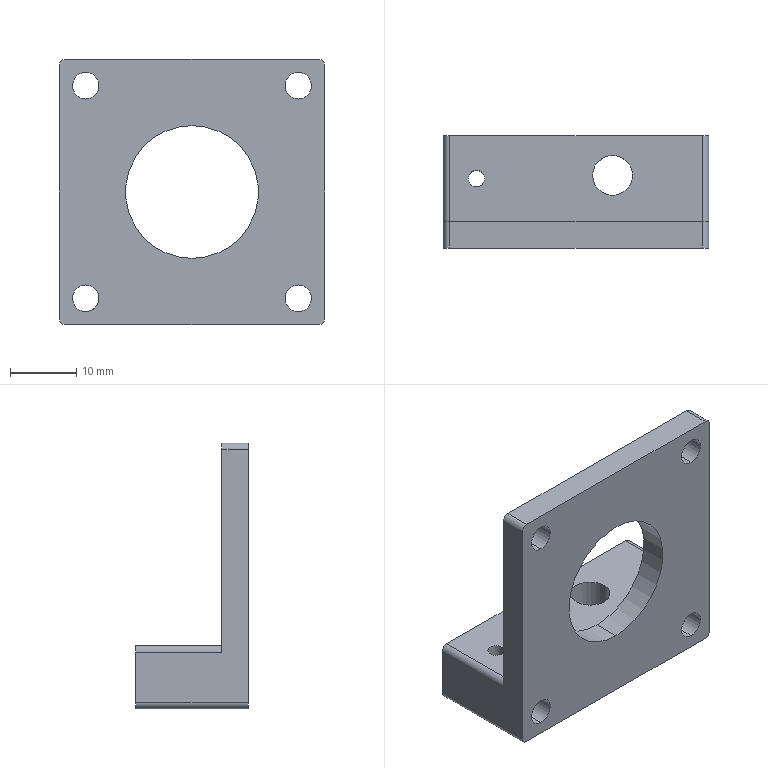Part | SolidWorks | features ICE 2, Extrusion 1, Fillet 1 | 1 solid | 29 faces | box 40 x 17 x 40 mm | volume 9241 mm3 | cylinder 21 | plane 8 | commonest cylinder face diameters 4 x9 2 x6 2.5 x2 6 x2 20 x2
STEP:
#1=CARTESIAN_POINT('',(-16.25,10.5,-40.));
#2=VERTEX_POINT('',#1);
#3=CARTESIAN_POINT('',(-13.75,10.5,-40.));
#4=VERTEX_POINT('',#3);
#5=CARTESIAN_POINT('',(-15.,10.5,-40.));
#6=DIRECTION('',(0.,0.,1.));
#7=DIRECTION('',(1.,0.,0.));
#8=AXIS2_PLACEMENT_3D('',#5,#6,#7);
#9=CIRCLE('',#8,1.25);
#10=EDGE_CURVE('',#2,#4,#9,.T.);
#11=ORIENTED_EDGE('',*,*,#10,.F.);
#12=CARTESIAN_POINT('',(-16.25,10.5,-37.984));
#13=VERTEX_POINT('',#12);
#14=CARTESIAN_POINT('',(-16.25,10.5,-40.));
#15=DIRECTION('',(0.,0.,1.));
#16=VECTOR('',#15,1000.);
#17=LINE('',#14,#16);
#18=EDGE_CURVE('',#2,#13,#17,.T.);
#19=ORIENTED_EDGE('',*,*,#18,.T.);
#20=CARTESIAN_POINT('',(-16.,9.75,-38.));
#21=VERTEX_POINT('',#20);
#22=CARTESIAN_POINT('',(-16.,9.75,-38.));
#23=CARTESIAN_POINT('',(-16.08,9.857,-38.));
#24=CARTESIAN_POINT('',(-16.144,9.978,-37.995));
#25=CARTESIAN_POINT('',(-16.228,10.232,-37.987));
#26=CARTESIAN_POINT('',(-16.25,10.366,-37.984));
#27=CARTESIAN_POINT('',(-16.25,10.5,-37.984));
#28=B_SPLINE_CURVE_WITH_KNOTS('',3,(#22,#23,#24,#25,#26,#27),.UNSPECIFIED.,.F.,.F.,(4,2,4),(0.006722,0.007123,0.007524),.UNSPECIFIED.);
#29=EDGE_CURVE('',#21,#13,#28,.T.);
#30=ORIENTED_EDGE('',*,*,#29,.F.);
#31=CARTESIAN_POINT('',(-16.,9.75,-34.));
#32=VERTEX_POINT('',#31);
#33=CARTESIAN_POINT('',(-16.,9.75,-34.));
#34=CARTESIAN_POINT('',(-15.915,9.636,-34.));
#35=CARTESIAN_POINT('',(-15.812,9.54,-34.005));
#36=CARTESIAN_POINT('',(-15.579,9.383,-34.041));
#37=CARTESIAN_POINT('',(-15.452,9.327,-34.072));
#38=CARTESIAN_POINT('',(-15.195,9.258,-34.164));
#39=CARTESIAN_POINT('',(-15.067,9.246,-34.226));
#40=CARTESIAN_POINT('',(-14.828,9.256,-34.374));
#41=CARTESIAN_POINT('',(-14.716,9.278,-34.46));
#42=CARTESIAN_POINT('',(-14.42,9.373,-34.743));
#43=CARTESIAN_POINT('',(-14.269,9.476,-34.964));
#44=CARTESIAN_POINT('',(-14.112,9.618,-35.327));
#45=CARTESIAN_POINT('',(-14.071,9.663,-35.456));
#46=CARTESIAN_POINT('',(-14.015,9.73,-35.722));
#47=CARTESIAN_POINT('',(-14.,9.75,-35.863));
#48=CARTESIAN_POINT('',(-14.,9.75,-36.143));
#49=CARTESIAN_POINT('',(-14.015,9.729,-36.282));
#50=CARTESIAN_POINT('',(-14.072,9.661,-36.549));
#51=CARTESIAN_POINT('',(-14.113,9.617,-36.675));
#52=CARTESIAN_POINT('',(-14.271,9.475,-37.039));
#53=CARTESIAN_POINT('',(-14.422,9.372,-37.259));
#54=CARTESIAN_POINT('',(-14.719,9.278,-37.542));
#55=CARTESIAN_POINT('',(-14.829,9.256,-37.627));
#56=CARTESIAN_POINT('',(-15.069,9.246,-37.776));
#57=CARTESIAN_POINT('',(-15.196,9.258,-37.836));
#58=CARTESIAN_POINT('',(-15.453,9.328,-37.929));
#59=CARTESIAN_POINT('',(-15.58,9.384,-37.959));
#60=CARTESIAN_POINT('',(-15.812,9.539,-37.995));
#61=CARTESIAN_POINT('',(-15.916,9.638,-38.));
#62=CARTESIAN_POINT('',(-16.,9.75,-38.));
#63=B_SPLINE_CURVE_WITH_KNOTS('',3,(#33,#34,#35,#36,#37,#38,#39,#40,#41,#42,#43,#44,#45,#46,#47,#48,#49,#50,#51,#52,#53,#54,#55,#56,#57,#58,#59,#60,#61,#62),.UNSPECIFIED.,.F.,.F.,(4,2,2,2,2,2,2,2,2,2,2,2,2,2,4),(0.,0.0004201,0.0008402,0.00126,0.00168,0.002521,0.002941,0.003361,0.003781,0.004201,0.005041,0.005462,0.005882,0.006302,0.006722),.UNSPECIFIED.);
#64=EDGE_CURVE('',#32,#21,#63,.T.);
#65=ORIENTED_EDGE('',*,*,#64,.F.);
#66=CARTESIAN_POINT('',(-16.25,10.5,-34.016));
#67=VERTEX_POINT('',#66);
#68=CARTESIAN_POINT('',(-16.25,10.5,-34.016));
#69=CARTESIAN_POINT('',(-16.25,10.366,-34.016));
#70=CARTESIAN_POINT('',(-16.228,10.233,-34.013));
#71=CARTESIAN_POINT('',(-16.144,9.978,-34.005));
#72=CARTESIAN_POINT('',(-16.081,9.858,-34.));
#73=CARTESIAN_POINT('',(-16.,9.75,-34.));
#74=B_SPLINE_CURVE_WITH_KNOTS('',3,(#68,#69,#70,#71,#72,#73),.UNSPECIFIED.,.F.,.F.,(4,2,4),(0.01585,0.01625,0.01665),.UNSPECIFIED.);
#75=EDGE_CURVE('',#67,#32,#74,.T.);
#76=ORIENTED_EDGE('',*,*,#75,.F.);
#77=CARTESIAN_POINT('',(-16.25,10.5,-30.5));
#78=VERTEX_POINT('',#77);
#79=CARTESIAN_POINT('',(-16.25,10.5,-40.));
#80=DIRECTION('',(0.,0.,1.));
#81=VECTOR('',#80,1000.);
#82=LINE('',#79,#81);
#83=EDGE_CURVE('',#67,#78,#82,.T.);
#84=ORIENTED_EDGE('',*,*,#83,.T.);
#85=CARTESIAN_POINT('',(-13.75,10.5,-30.5));
#86=VERTEX_POINT('',#85);
#87=CARTESIAN_POINT('',(-15.,10.5,-30.5));
#88=DIRECTION('',(0.,0.,1.));
#89=DIRECTION('',(1.,0.,0.));
#90=AXIS2_PLACEMENT_3D('',#87,#88,#89);
#91=CIRCLE('',#90,1.25);
#92=EDGE_CURVE('',#78,#86,#91,.T.);
#93=ORIENTED_EDGE('',*,*,#92,.T.);
#94=CARTESIAN_POINT('',(-13.75,10.5,-40.));
#95=DIRECTION('',(0.,0.,1.));
#96=VECTOR('',#95,1000.);
#97=LINE('',#94,#96);
#98=EDGE_CURVE('',#4,#86,#97,.T.);
#99=ORIENTED_EDGE('',*,*,#98,.F.);
#100=EDGE_LOOP('',(#11,#19,#30,#65,#76,#84,#93,#99));
#101=FACE_OUTER_BOUND('',#100,.T.);
#102=CARTESIAN_POINT('',(-15.,10.5,-40.));
#103=DIRECTION('',(0.,0.,1.));
#104=DIRECTION('',(1.,0.,0.));
#105=AXIS2_PLACEMENT_3D('',#102,#103,#104);
#106=CYLINDRICAL_SURFACE('',#105,1.25);
#107=ADVANCED_FACE('',(#101),#106,.F.);
#108=CARTESIAN_POINT('',(2.5,11.,-40.));
#109=VERTEX_POINT('',#108);
#110=CARTESIAN_POINT('',(8.5,11.,-40.));
#111=VERTEX_POINT('',#110);
#112=CARTESIAN_POINT('',(5.5,11.,-40.));
#113=DIRECTION('',(0.,0.,1.));
#114=DIRECTION('',(1.,0.,0.));
#115=AXIS2_PLACEMENT_3D('',#112,#113,#114);
#116=CIRCLE('',#115,3.);
#117=EDGE_CURVE('',#109,#111,#116,.T.);
#118=ORIENTED_EDGE('',*,*,#117,.F.);
#119=CARTESIAN_POINT('',(2.5,11.,-30.5));
#120=VERTEX_POINT('',#119);
#121=CARTESIAN_POINT('',(2.5,11.,-40.));
#122=DIRECTION('',(0.,0.,1.));
#123=VECTOR('',#122,1000.);
#124=LINE('',#121,#123);
#125=EDGE_CURVE('',#109,#120,#124,.T.);
#126=ORIENTED_EDGE('',*,*,#125,.T.);
#127=CARTESIAN_POINT('',(8.5,11.,-30.5));
#128=VERTEX_POINT('',#127);
#129=CARTESIAN_POINT('',(5.5,11.,-30.5));
#130=DIRECTION('',(0.,0.,1.));
#131=DIRECTION('',(1.,0.,0.));
#132=AXIS2_PLACEMENT_3D('',#129,#130,#131);
#133=CIRCLE('',#132,3.);
#134=EDGE_CURVE('',#120,#128,#133,.T.);
#135=ORIENTED_EDGE('',*,*,#134,.T.);
#136=CARTESIAN_POINT('',(8.5,11.,-40.));
#137=DIRECTION('',(0.,0.,1.));
#138=VECTOR('',#137,1000.);
#139=LINE('',#136,#138);
#140=EDGE_CURVE('',#111,#128,#139,.T.);
#141=ORIENTED_EDGE('',*,*,#140,.F.);
#142=EDGE_LOOP('',(#118,#126,#135,#141));
#143=FACE_OUTER_BOUND('',#142,.T.);
#144=CARTESIAN_POINT('',(5.5,11.,-40.));
#145=DIRECTION('',(0.,0.,1.));
#146=DIRECTION('',(1.,0.,0.));
#147=AXIS2_PLACEMENT_3D('',#144,#145,#146);
#148=CYLINDRICAL_SURFACE('',#147,3.);
#149=ADVANCED_FACE('',(#143),#148,.F.);
#150=CARTESIAN_POINT('',(-16.,0.,-38.));
#151=VERTEX_POINT('',#150);
#152=CARTESIAN_POINT('',(-16.,0.,-34.));
#153=VERTEX_POINT('',#152);
#154=CARTESIAN_POINT('',(-16.,0.,-36.));
#155=DIRECTION('',(0.,1.,0.));
#156=DIRECTION('',(0.,0.,1.));
#157=AXIS2_PLACEMENT_3D('',#154,#155,#156);
#158=CIRCLE('',#157,2.);
#159=EDGE_CURVE('',#151,#153,#158,.T.);
#160=ORIENTED_EDGE('',*,*,#159,.F.);
#161=CARTESIAN_POINT('',(-16.,0.,-38.));
#162=DIRECTION('',(0.,1.,0.));
#163=VECTOR('',#162,1000.);
#164=LINE('',#161,#163);
#165=EDGE_CURVE('',#151,#21,#164,.T.);
#166=ORIENTED_EDGE('',*,*,#165,.T.);
#167=ORIENTED_EDGE('',*,*,#29,.T.);
#168=CARTESIAN_POINT('',(-16.,11.25,-38.));
#169=VERTEX_POINT('',#168);
#170=CARTESIAN_POINT('',(-16.25,10.5,-37.984));
#171=CARTESIAN_POINT('',(-16.25,10.634,-37.984));
#172=CARTESIAN_POINT('',(-16.228,10.768,-37.987));
#173=CARTESIAN_POINT('',(-16.143,11.022,-37.995));
#174=CARTESIAN_POINT('',(-16.081,11.143,-38.));
#175=CARTESIAN_POINT('',(-16.,11.25,-38.));
#176=B_SPLINE_CURVE_WITH_KNOTS('',3,(#170,#171,#172,#173,#174,#175),.UNSPECIFIED.,.F.,.F.,(4,2,4),(0.007524,0.007925,0.008326),.UNSPECIFIED.);
#177=EDGE_CURVE('',#13,#169,#176,.T.);
#178=ORIENTED_EDGE('',*,*,#177,.T.);
#179=CARTESIAN_POINT('',(-16.,17.,-38.));
#180=VERTEX_POINT('',#179);
#181=CARTESIAN_POINT('',(-16.,0.,-38.));
#182=DIRECTION('',(0.,1.,0.));
#183=VECTOR('',#182,1000.);
#184=LINE('',#181,#183);
#185=EDGE_CURVE('',#169,#180,#184,.T.);
#186=ORIENTED_EDGE('',*,*,#185,.T.);
#187=CARTESIAN_POINT('',(-16.,17.,-34.));
#188=VERTEX_POINT('',#187);
#189=CARTESIAN_POINT('',(-16.,17.,-36.));
#190=DIRECTION('',(0.,1.,0.));
#191=DIRECTION('',(0.,0.,1.));
#192=AXIS2_PLACEMENT_3D('',#189,#190,#191);
#193=CIRCLE('',#192,2.);
#194=EDGE_CURVE('',#180,#188,#193,.T.);
#195=ORIENTED_EDGE('',*,*,#194,.T.);
#196=CARTESIAN_POINT('',(-16.,11.25,-34.));
#197=VERTEX_POINT('',#196);
#198=CARTESIAN_POINT('',(-16.,0.,-34.));
#199=DIRECTION('',(0.,1.,0.));
#200=VECTOR('',#199,1000.);
#201=LINE('',#198,#200);
#202=EDGE_CURVE('',#197,#188,#201,.T.);
#203=ORIENTED_EDGE('',*,*,#202,.F.);
#204=CARTESIAN_POINT('',(-16.,11.25,-34.));
#205=CARTESIAN_POINT('',(-16.081,11.142,-34.));
#206=CARTESIAN_POINT('',(-16.143,11.023,-34.005));
#207=CARTESIAN_POINT('',(-16.229,10.767,-34.013));
#208=CARTESIAN_POINT('',(-16.25,10.635,-34.016));
#209=CARTESIAN_POINT('',(-16.25,10.5,-34.016));
#210=B_SPLINE_CURVE_WITH_KNOTS('',3,(#204,#205,#206,#207,#208,#209),.UNSPECIFIED.,.F.,.F.,(4,2,4),(0.01505,0.01545,0.01585),.UNSPECIFIED.);
#211=EDGE_CURVE('',#197,#67,#210,.T.);
#212=ORIENTED_EDGE('',*,*,#211,.T.);
#213=ORIENTED_EDGE('',*,*,#75,.T.);
#214=CARTESIAN_POINT('',(-16.,0.,-34.));
#215=DIRECTION('',(0.,1.,0.));
#216=VECTOR('',#215,1000.);
#217=LINE('',#214,#216);
#218=EDGE_CURVE('',#153,#32,#217,.T.);
#219=ORIENTED_EDGE('',*,*,#218,.F.);
#220=EDGE_LOOP('',(#160,#166,#167,#178,#186,#195,#203,#212,#213,#219));
#221=FACE_OUTER_BOUND('',#220,.T.);
#222=CARTESIAN_POINT('',(-16.,0.,-36.));
#223=DIRECTION('',(0.,1.,0.));
#224=DIRECTION('',(0.,0.,1.));
#225=AXIS2_PLACEMENT_3D('',#222,#223,#224);
#226=CYLINDRICAL_SURFACE('',#225,2.);
#227=ADVANCED_FACE('',(#221),#226,.F.);
#228=ORIENTED_EDGE('',*,*,#165,.F.);
#229=CARTESIAN_POINT('',(-16.,0.,-36.));
#230=DIRECTION('',(0.,1.,0.));
#231=DIRECTION('',(0.,0.,1.));
#232=AXIS2_PLACEMENT_3D('',#229,#230,#231);
#233=CIRCLE('',#232,2.);
#234=EDGE_CURVE('',#153,#151,#233,.T.);
#235=ORIENTED_EDGE('',*,*,#234,.F.);
#236=ORIENTED_EDGE('',*,*,#218,.T.);
#237=ORIENTED_EDGE('',*,*,#64,.T.);
#238=EDGE_LOOP('',(#228,#235,#236,#237));
#239=FACE_OUTER_BOUND('',#238,.T.);
#240=CARTESIAN_POINT('',(-16.,0.,-36.));
#241=DIRECTION('',(0.,1.,0.));
#242=DIRECTION('',(0.,0.,1.));
#243=AXIS2_PLACEMENT_3D('',#240,#241,#242);
#244=CYLINDRICAL_SURFACE('',#243,2.);
#245=ADVANCED_FACE('',(#239),#244,.F.);
#246=CARTESIAN_POINT('',(-16.,0.,-6.));
#247=VERTEX_POINT('',#246);
#248=CARTESIAN_POINT('',(-16.,0.,-2.));
#249=VERTEX_POINT('',#248);
#250=CARTESIAN_POINT('',(-16.,0.,-4.));
#251=DIRECTION('',(0.,1.,0.));
#252=DIRECTION('',(0.,0.,1.));
#253=AXIS2_PLACEMENT_3D('',#250,#251,#252);
#254=CIRCLE('',#253,2.);
#255=EDGE_CURVE('',#247,#249,#254,.T.);
#256=ORIENTED_EDGE('',*,*,#255,.F.);
#257=CARTESIAN_POINT('',(-16.,4.,-6.));
#258=VERTEX_POINT('',#257);
#259=CARTESIAN_POINT('',(-16.,0.,-6.));
#260=DIRECTION('',(0.,1.,0.));
#261=VECTOR('',#260,1000.);
#262=LINE('',#259,#261);
#263=EDGE_CURVE('',#247,#258,#262,.T.);
#264=ORIENTED_EDGE('',*,*,#263,.T.);
#265=CARTESIAN_POINT('',(-16.,4.,-2.));
#266=VERTEX_POINT('',#265);
#267=CARTESIAN_POINT('',(-16.,4.,-4.));
#268=DIRECTION('',(0.,-1.,0.));
#269=DIRECTION('',(0.,0.,-1.));
#270=AXIS2_PLACEMENT_3D('',#267,#268,#269);
#271=CIRCLE('',#270,2.);
#272=EDGE_CURVE('',#266,#258,#271,.T.);
#273=ORIENTED_EDGE('',*,*,#272,.F.);
#274=CARTESIAN_POINT('',(-16.,0.,-2.));
#275=DIRECTION('',(0.,1.,0.));
#276=VECTOR('',#275,1000.);
#277=LINE('',#274,#276);
#278=EDGE_CURVE('',#249,#266,#277,.T.);
#279=ORIENTED_EDGE('',*,*,#278,.F.);
#280=EDGE_LOOP('',(#256,#264,#273,#279));
#281=FACE_OUTER_BOUND('',#280,.T.);
#282=CARTESIAN_POINT('',(-16.,0.,-4.));
#283=DIRECTION('',(0.,1.,0.));
#284=DIRECTION('',(0.,0.,1.));
#285=AXIS2_PLACEMENT_3D('',#282,#283,#284);
#286=CYLINDRICAL_SURFACE('',#285,2.);
#287=ADVANCED_FACE('',(#281),#286,.F.);
#288=CARTESIAN_POINT('',(16.,0.,-6.));
#289=VERTEX_POINT('',#288);
#290=CARTESIAN_POINT('',(16.,0.,-2.));
#291=VERTEX_POINT('',#290);
#292=CARTESIAN_POINT('',(16.,0.,-4.));
#293=DIRECTION('',(0.,1.,0.));
#294=DIRECTION('',(0.,0.,1.));
#295=AXIS2_PLACEMENT_3D('',#292,#293,#294);
#296=CIRCLE('',#295,2.);
#297=EDGE_CURVE('',#289,#291,#296,.T.);
#298=ORIENTED_EDGE('',*,*,#297,.F.);
#299=CARTESIAN_POINT('',(16.,4.,-6.));
#300=VERTEX_POINT('',#299);
#301=CARTESIAN_POINT('',(16.,0.,-6.));
#302=DIRECTION('',(0.,1.,0.));
#303=VECTOR('',#302,1000.);
#304=LINE('',#301,#303);
#305=EDGE_CURVE('',#289,#300,#304,.T.);
#306=ORIENTED_EDGE('',*,*,#305,.T.);
#307=CARTESIAN_POINT('',(16.,4.,-2.));
#308=VERTEX_POINT('',#307);
#309=CARTESIAN_POINT('',(16.,4.,-4.));
#310=DIRECTION('',(0.,-1.,0.));
#311=DIRECTION('',(0.,0.,-1.));
#312=AXIS2_PLACEMENT_3D('',#309,#310,#311);
#313=CIRCLE('',#312,2.);
#314=EDGE_CURVE('',#308,#300,#313,.T.);
#315=ORIENTED_EDGE('',*,*,#314,.F.);
#316=CARTESIAN_POINT('',(16.,0.,-2.));
#317=DIRECTION('',(0.,1.,0.));
#318=VECTOR('',#317,1000.);
#319=LINE('',#316,#318);
#320=EDGE_CURVE('',#291,#308,#319,.T.);
#321=ORIENTED_EDGE('',*,*,#320,.F.);
#322=EDGE_LOOP('',(#298,#306,#315,#321));
#323=FACE_OUTER_BOUND('',#322,.T.);
#324=CARTESIAN_POINT('',(16.,0.,-4.));
#325=DIRECTION('',(0.,1.,0.));
#326=DIRECTION('',(0.,0.,1.));
#327=AXIS2_PLACEMENT_3D('',#324,#325,#326);
#328=CYLINDRICAL_SURFACE('',#327,2.);
#329=ADVANCED_FACE('',(#323),#328,.F.);
#330=CARTESIAN_POINT('',(16.,0.,-38.));
#331=VERTEX_POINT('',#330);
#332=CARTESIAN_POINT('',(16.,0.,-34.));
#333=VERTEX_POINT('',#332);
#334=CARTESIAN_POINT('',(16.,0.,-36.));
#335=DIRECTION('',(0.,1.,0.));
#336=DIRECTION('',(0.,0.,1.));
#337=AXIS2_PLACEMENT_3D('',#334,#335,#336);
#338=CIRCLE('',#337,2.);
#339=EDGE_CURVE('',#331,#333,#338,.T.);
#340=ORIENTED_EDGE('',*,*,#339,.F.);
#341=CARTESIAN_POINT('',(16.,17.,-38.));
#342=VERTEX_POINT('',#341);
#343=CARTESIAN_POINT('',(16.,0.,-38.));
#344=DIRECTION('',(0.,1.,0.));
#345=VECTOR('',#344,1000.);
#346=LINE('',#343,#345);
#347=EDGE_CURVE('',#331,#342,#346,.T.);
#348=ORIENTED_EDGE('',*,*,#347,.T.);
#349=CARTESIAN_POINT('',(16.,17.,-34.));
#350=VERTEX_POINT('',#349);
#351=CARTESIAN_POINT('',(16.,17.,-36.));
#352=DIRECTION('',(0.,1.,0.));
#353=DIRECTION('',(0.,0.,1.));
#354=AXIS2_PLACEMENT_3D('',#351,#352,#353);
#355=CIRCLE('',#354,2.);
#356=EDGE_CURVE('',#342,#350,#355,.T.);
#357=ORIENTED_EDGE('',*,*,#356,.T.);
#358=CARTESIAN_POINT('',(16.,0.,-34.));
#359=DIRECTION('',(0.,1.,0.));
#360=VECTOR('',#359,1000.);
#361=LINE('',#358,#360);
#362=EDGE_CURVE('',#333,#350,#361,.T.);
#363=ORIENTED_EDGE('',*,*,#362,.F.);
#364=EDGE_LOOP('',(#340,#348,#357,#363));
#365=FACE_OUTER_BOUND('',#364,.T.);
#366=CARTESIAN_POINT('',(16.,0.,-36.));
#367=DIRECTION('',(0.,1.,0.));
#368=DIRECTION('',(0.,0.,1.));
#369=AXIS2_PLACEMENT_3D('',#366,#367,#368);
#370=CYLINDRICAL_SURFACE('',#369,2.);
#371=ADVANCED_FACE('',(#365),#370,.F.);
#372=CARTESIAN_POINT('',(0.,0.,-30.));
#373=VERTEX_POINT('',#372);
#374=CARTESIAN_POINT('',(0.,0.,-10.));
#375=VERTEX_POINT('',#374);
#376=CARTESIAN_POINT('',(0.,0.,-20.));
#377=DIRECTION('',(0.,1.,0.));
#378=DIRECTION('',(0.,0.,1.));
#379=AXIS2_PLACEMENT_3D('',#376,#377,#378);
#380=CIRCLE('',#379,10.);
#381=EDGE_CURVE('',#373,#375,#380,.T.);
#382=ORIENTED_EDGE('',*,*,#381,.F.);
#383=CARTESIAN_POINT('',(0.,4.,-30.));
#384=VERTEX_POINT('',#383);
#385=CARTESIAN_POINT('',(0.,0.,-30.));
#386=DIRECTION('',(0.,1.,0.));
#387=VECTOR('',#386,1000.);
#388=LINE('',#385,#387);
#389=EDGE_CURVE('',#373,#384,#388,.T.);
#390=ORIENTED_EDGE('',*,*,#389,.T.);
#391=CARTESIAN_POINT('',(0.,4.,-10.));
#392=VERTEX_POINT('',#391);
#393=CARTESIAN_POINT('',(0.,4.,-20.));
#394=DIRECTION('',(0.,-1.,0.));
#395=DIRECTION('',(0.,0.,-1.));
#396=AXIS2_PLACEMENT_3D('',#393,#394,#395);
#397=CIRCLE('',#396,10.);
#398=EDGE_CURVE('',#392,#384,#397,.T.);
#399=ORIENTED_EDGE('',*,*,#398,.F.);
#400=CARTESIAN_POINT('',(0.,0.,-10.));
#401=DIRECTION('',(0.,1.,0.));
#402=VECTOR('',#401,1000.);
#403=LINE('',#400,#402);
#404=EDGE_CURVE('',#375,#392,#403,.T.);
#405=ORIENTED_EDGE('',*,*,#404,.F.);
#406=EDGE_LOOP('',(#382,#390,#399,#405));
#407=FACE_OUTER_BOUND('',#406,.T.);
#408=CARTESIAN_POINT('',(0.,0.,-20.));
#409=DIRECTION('',(0.,1.,0.));
#410=DIRECTION('',(0.,0.,1.));
#411=AXIS2_PLACEMENT_3D('',#408,#409,#410);
#412=CYLINDRICAL_SURFACE('',#411,10.);
#413=ADVANCED_FACE('',(#407),#412,.F.);
#414=CARTESIAN_POINT('',(19.,4.,0.));
#415=VERTEX_POINT('',#414);
#416=CARTESIAN_POINT('',(-19.,4.,0.));
#417=VERTEX_POINT('',#416);
#418=CARTESIAN_POINT('',(20.,4.,0.));
#419=DIRECTION('',(-1.,0.,0.));
#420=VECTOR('',#419,1000.);
#421=LINE('',#418,#420);
#422=EDGE_CURVE('',#415,#417,#421,.T.);
#423=ORIENTED_EDGE('',*,*,#422,.T.);
#424=CARTESIAN_POINT('',(-19.,0.,0.));
#425=VERTEX_POINT('',#424);
#426=CARTESIAN_POINT('',(-19.,0.,0.));
#427=DIRECTION('',(0.,-1.,0.));
#428=VECTOR('',#427,1000.);
#429=LINE('',#426,#428);
#430=EDGE_CURVE('',#417,#425,#429,.T.);
#431=ORIENTED_EDGE('',*,*,#430,.T.);
#432=CARTESIAN_POINT('',(19.,0.,0.));
#433=VERTEX_POINT('',#432);
#434=CARTESIAN_POINT('',(20.,0.,0.));
#435=DIRECTION('',(-1.,0.,0.));
#436=VECTOR('',#435,1000.);
#437=LINE('',#434,#436);
#438=EDGE_CURVE('',#433,#425,#437,.T.);
#439=ORIENTED_EDGE('',*,*,#438,.F.);
#440=CARTESIAN_POINT('',(19.,0.,0.));
#441=DIRECTION('',(0.,1.,0.));
#442=VECTOR('',#441,1000.);
#443=LINE('',#440,#442);
#444=EDGE_CURVE('',#433,#415,#443,.T.);
#445=ORIENTED_EDGE('',*,*,#444,.T.);
#446=EDGE_LOOP('',(#423,#431,#439,#445));
#447=FACE_OUTER_BOUND('',#446,.T.);
#448=CARTESIAN_POINT('',(20.,0.,0.));
#449=DIRECTION('',(0.,0.,-1.));
#450=DIRECTION('',(-1.,0.,0.));
#451=AXIS2_PLACEMENT_3D('',#448,#449,#450);
#452=PLANE('',#451);
#453=ADVANCED_FACE('',(#447),#452,.F.);
#454=ORIENTED_EDGE('',*,*,#234,.T.);
#455=ORIENTED_EDGE('',*,*,#159,.T.);
#456=EDGE_LOOP('',(#454,#455));
#457=FACE_BOUND('',#456,.T.);
#458=CARTESIAN_POINT('',(-16.,0.,-4.));
#459=DIRECTION('',(0.,1.,0.));
#460=DIRECTION('',(0.,0.,1.));
#461=AXIS2_PLACEMENT_3D('',#458,#459,#460);
#462=CIRCLE('',#461,2.);
#463=EDGE_CURVE('',#249,#247,#462,.T.);
#464=ORIENTED_EDGE('',*,*,#463,.T.);
#465=ORIENTED_EDGE('',*,*,#255,.T.);
#466=EDGE_LOOP('',(#464,#465));
#467=FACE_BOUND('',#466,.T.);
#468=CARTESIAN_POINT('',(16.,0.,-4.));
#469=DIRECTION('',(0.,1.,0.));
#470=DIRECTION('',(0.,0.,1.));
#471=AXIS2_PLACEMENT_3D('',#468,#469,#470);
#472=CIRCLE('',#471,2.);
#473=EDGE_CURVE('',#291,#289,#472,.T.);
#474=ORIENTED_EDGE('',*,*,#473,.T.);
#475=ORIENTED_EDGE('',*,*,#297,.T.);
#476=EDGE_LOOP('',(#474,#475));
#477=FACE_BOUND('',#476,.T.);
#478=CARTESIAN_POINT('',(16.,0.,-36.));
#479=DIRECTION('',(0.,1.,0.));
#480=DIRECTION('',(0.,0.,1.));
#481=AXIS2_PLACEMENT_3D('',#478,#479,#480);
#482=CIRCLE('',#481,2.);
#483=EDGE_CURVE('',#333,#331,#482,.T.);
#484=ORIENTED_EDGE('',*,*,#483,.T.);
#485=ORIENTED_EDGE('',*,*,#339,.T.);
#486=EDGE_LOOP('',(#484,#485));
#487=FACE_BOUND('',#486,.T.);
#488=CARTESIAN_POINT('',(0.,0.,-20.));
#489=DIRECTION('',(0.,1.,0.));
#490=DIRECTION('',(0.,0.,1.));
#491=AXIS2_PLACEMENT_3D('',#488,#489,#490);
#492=CIRCLE('',#491,10.);
#493=EDGE_CURVE('',#375,#373,#492,.T.);
#494=ORIENTED_EDGE('',*,*,#493,.T.);
#495=ORIENTED_EDGE('',*,*,#381,.T.);
#496=EDGE_LOOP('',(#494,#495));
#497=FACE_BOUND('',#496,.T.);
#498=ORIENTED_EDGE('',*,*,#438,.T.);
#499=CARTESIAN_POINT('',(-20.,0.,-1.));
#500=VERTEX_POINT('',#499);
#501=CARTESIAN_POINT('',(-19.,0.,-1.));
#502=DIRECTION('',(0.,-1.,0.));
#503=DIRECTION('',(0.,0.,1.));
#504=AXIS2_PLACEMENT_3D('',#501,#502,#503);
#505=CIRCLE('',#504,1.);
#506=EDGE_CURVE('',#425,#500,#505,.T.);
#507=ORIENTED_EDGE('',*,*,#506,.T.);
#508=CARTESIAN_POINT('',(-20.,0.,-39.));
#509=VERTEX_POINT('',#508);
#510=CARTESIAN_POINT('',(-20.,0.,0.));
#511=DIRECTION('',(0.,0.,-1.));
#512=VECTOR('',#511,1000.);
#513=LINE('',#510,#512);
#514=EDGE_CURVE('',#500,#509,#513,.T.);
#515=ORIENTED_EDGE('',*,*,#514,.T.);
#516=CARTESIAN_POINT('',(-19.,0.,-40.));
#517=VERTEX_POINT('',#516);
#518=CARTESIAN_POINT('',(-19.,0.,-39.));
#519=DIRECTION('',(0.,-1.,0.));
#520=DIRECTION('',(0.,0.,1.));
#521=AXIS2_PLACEMENT_3D('',#518,#519,#520);
#522=CIRCLE('',#521,1.);
#523=EDGE_CURVE('',#509,#517,#522,.T.);
#524=ORIENTED_EDGE('',*,*,#523,.T.);
#525=CARTESIAN_POINT('',(19.,0.,-40.));
#526=VERTEX_POINT('',#525);
#527=CARTESIAN_POINT('',(20.,0.,-40.));
#528=DIRECTION('',(-1.,0.,0.));
#529=VECTOR('',#528,1000.);
#530=LINE('',#527,#529);
#531=EDGE_CURVE('',#526,#517,#530,.T.);
#532=ORIENTED_EDGE('',*,*,#531,.F.);
#533=CARTESIAN_POINT('',(20.,0.,-39.));
#534=VERTEX_POINT('',#533);
#535=CARTESIAN_POINT('',(19.,0.,-39.));
#536=DIRECTION('',(0.,-1.,0.));
#537=DIRECTION('',(0.,0.,1.));
#538=AXIS2_PLACEMENT_3D('',#535,#536,#537);
#539=CIRCLE('',#538,1.);
#540=EDGE_CURVE('',#526,#534,#539,.T.);
#541=ORIENTED_EDGE('',*,*,#540,.T.);
#542=CARTESIAN_POINT('',(20.,0.,-1.));
#543=VERTEX_POINT('',#542);
#544=CARTESIAN_POINT('',(20.,0.,0.));
#545=DIRECTION('',(0.,0.,-1.));
#546=VECTOR('',#545,1000.);
#547=LINE('',#544,#546);
#548=EDGE_CURVE('',#543,#534,#547,.T.);
#549=ORIENTED_EDGE('',*,*,#548,.F.);
#550=CARTESIAN_POINT('',(19.,0.,-1.));
#551=DIRECTION('',(0.,-1.,0.));
#552=DIRECTION('',(0.,0.,1.));
#553=AXIS2_PLACEMENT_3D('',#550,#551,#552);
#554=CIRCLE('',#553,1.);
#555=EDGE_CURVE('',#543,#433,#554,.T.);
#556=ORIENTED_EDGE('',*,*,#555,.T.);
#557=EDGE_LOOP('',(#498,#507,#515,#524,#532,#541,#549,#556));
#558=FACE_OUTER_BOUND('',#557,.T.);
#559=CARTESIAN_POINT('',(20.,0.,0.));
#560=DIRECTION('',(0.,1.,0.));
#561=DIRECTION('',(0.,0.,1.));
#562=AXIS2_PLACEMENT_3D('',#559,#560,#561);
#563=PLANE('',#562);
#564=ADVANCED_FACE('',(#457,#467,#477,#487,#497,#558),#563,.F.);
#565=CARTESIAN_POINT('',(-15.,10.5,-40.));
#566=DIRECTION('',(0.,0.,1.));
#567=DIRECTION('',(1.,0.,0.));
#568=AXIS2_PLACEMENT_3D('',#565,#566,#567);
#569=CIRCLE('',#568,1.25);
#570=EDGE_CURVE('',#4,#2,#569,.T.);
#571=ORIENTED_EDGE('',*,*,#570,.T.);
#572=ORIENTED_EDGE('',*,*,#10,.T.);
#573=EDGE_LOOP('',(#571,#572));
#574=FACE_BOUND('',#573,.T.);
#575=CARTESIAN_POINT('',(5.5,11.,-40.));
#576=DIRECTION('',(0.,0.,1.));
#577=DIRECTION('',(1.,0.,0.));
#578=AXIS2_PLACEMENT_3D('',#575,#576,#577);
#579=CIRCLE('',#578,3.);
#580=EDGE_CURVE('',#111,#109,#579,.T.);
#581=ORIENTED_EDGE('',*,*,#580,.T.);
#582=ORIENTED_EDGE('',*,*,#117,.T.);
#583=EDGE_LOOP('',(#581,#582));
#584=FACE_BOUND('',#583,.T.);
#585=ORIENTED_EDGE('',*,*,#531,.T.);
#586=CARTESIAN_POINT('',(-19.,17.,-40.));
#587=VERTEX_POINT('',#586);
#588=CARTESIAN_POINT('',(-19.,17.,-40.));
#589=DIRECTION('',(0.,1.,0.));
#590=VECTOR('',#589,1000.);
#591=LINE('',#588,#590);
#592=EDGE_CURVE('',#517,#587,#591,.T.);
#593=ORIENTED_EDGE('',*,*,#592,.T.);
#594=CARTESIAN_POINT('',(19.,17.,-40.));
#595=VERTEX_POINT('',#594);
#596=CARTESIAN_POINT('',(20.,17.,-40.));
#597=DIRECTION('',(-1.,0.,0.));
#598=VECTOR('',#597,1000.);
#599=LINE('',#596,#598);
#600=EDGE_CURVE('',#595,#587,#599,.T.);
#601=ORIENTED_EDGE('',*,*,#600,.F.);
#602=CARTESIAN_POINT('',(19.,4.,-40.));
#603=DIRECTION('',(0.,-1.,0.));
#604=VECTOR('',#603,1000.);
#605=LINE('',#602,#604);
#606=EDGE_CURVE('',#595,#526,#605,.T.);
#607=ORIENTED_EDGE('',*,*,#606,.T.);
#608=EDGE_LOOP('',(#585,#593,#601,#607));
#609=FACE_OUTER_BOUND('',#608,.T.);
#610=CARTESIAN_POINT('',(20.,4.,-40.));
#611=DIRECTION('',(0.,0.,1.));
#612=DIRECTION('',(1.,0.,0.));
#613=AXIS2_PLACEMENT_3D('',#610,#611,#612);
#614=PLANE('',#613);
#615=ADVANCED_FACE('',(#574,#584,#609),#614,.F.);
#616=CARTESIAN_POINT('',(-16.,17.,-36.));
#617=DIRECTION('',(0.,1.,0.));
#618=DIRECTION('',(0.,0.,1.));
#619=AXIS2_PLACEMENT_3D('',#616,#617,#618);
#620=CIRCLE('',#619,2.);
#621=EDGE_CURVE('',#188,#180,#620,.T.);
#622=ORIENTED_EDGE('',*,*,#621,.F.);
#623=ORIENTED_EDGE('',*,*,#194,.F.);
#624=EDGE_LOOP('',(#622,#623));
#625=FACE_BOUND('',#624,.T.);
#626=CARTESIAN_POINT('',(16.,17.,-36.));
#627=DIRECTION('',(0.,1.,0.));
#628=DIRECTION('',(0.,0.,1.));
#629=AXIS2_PLACEMENT_3D('',#626,#627,#628);
#630=CIRCLE('',#629,2.);
#631=EDGE_CURVE('',#350,#342,#630,.T.);
#632=ORIENTED_EDGE('',*,*,#631,.F.);
#633=ORIENTED_EDGE('',*,*,#356,.F.);
#634=EDGE_LOOP('',(#632,#633));
#635=FACE_BOUND('',#634,.T.);
#636=ORIENTED_EDGE('',*,*,#600,.T.);
#637=CARTESIAN_POINT('',(-20.,17.,-39.));
#638=VERTEX_POINT('',#637);
#639=CARTESIAN_POINT('',(-19.,17.,-39.));
#640=DIRECTION('',(0.,1.,0.));
#641=DIRECTION('',(0.,0.,-1.));
#642=AXIS2_PLACEMENT_3D('',#639,#640,#641);
#643=CIRCLE('',#642,1.);
#644=EDGE_CURVE('',#587,#638,#643,.T.);
#645=ORIENTED_EDGE('',*,*,#644,.T.);
#646=CARTESIAN_POINT('',(-20.,17.,-31.5));
#647=VERTEX_POINT('',#646);
#648=CARTESIAN_POINT('',(-20.,17.,-40.));
#649=DIRECTION('',(0.,0.,1.));
#650=VECTOR('',#649,1000.);
#651=LINE('',#648,#650);
#652=EDGE_CURVE('',#638,#647,#651,.T.);
#653=ORIENTED_EDGE('',*,*,#652,.T.);
#654=CARTESIAN_POINT('',(-19.,17.,-30.5));
#655=VERTEX_POINT('',#654);
#656=CARTESIAN_POINT('',(-19.,17.,-31.5));
#657=DIRECTION('',(0.,1.,0.));
#658=DIRECTION('',(0.,0.,-1.));
#659=AXIS2_PLACEMENT_3D('',#656,#657,#658);
#660=CIRCLE('',#659,1.);
#661=EDGE_CURVE('',#647,#655,#660,.T.);
#662=ORIENTED_EDGE('',*,*,#661,.T.);
#663=CARTESIAN_POINT('',(19.,17.,-30.5));
#664=VERTEX_POINT('',#663);
#665=CARTESIAN_POINT('',(20.,17.,-30.5));
#666=DIRECTION('',(-1.,0.,0.));
#667=VECTOR('',#666,1000.);
#668=LINE('',#665,#667);
#669=EDGE_CURVE('',#664,#655,#668,.T.);
#670=ORIENTED_EDGE('',*,*,#669,.F.);
#671=CARTESIAN_POINT('',(20.,17.,-31.5));
#672=VERTEX_POINT('',#671);
#673=CARTESIAN_POINT('',(19.,17.,-31.5));
#674=DIRECTION('',(0.,1.,0.));
#675=DIRECTION('',(0.,0.,-1.));
#676=AXIS2_PLACEMENT_3D('',#673,#674,#675);
#677=CIRCLE('',#676,1.);
#678=EDGE_CURVE('',#664,#672,#677,.T.);
#679=ORIENTED_EDGE('',*,*,#678,.T.);
#680=CARTESIAN_POINT('',(20.,17.,-39.));
#681=VERTEX_POINT('',#680);
#682=CARTESIAN_POINT('',(20.,17.,-40.));
#683=DIRECTION('',(0.,0.,1.));
#684=VECTOR('',#683,1000.);
#685=LINE('',#682,#684);
#686=EDGE_CURVE('',#681,#672,#685,.T.);
#687=ORIENTED_EDGE('',*,*,#686,.F.);
#688=CARTESIAN_POINT('',(19.,17.,-39.));
#689=DIRECTION('',(0.,1.,0.));
#690=DIRECTION('',(0.,0.,-1.));
#691=AXIS2_PLACEMENT_3D('',#688,#689,#690);
#692=CIRCLE('',#691,1.);
#693=EDGE_CURVE('',#681,#595,#692,.T.);
#694=ORIENTED_EDGE('',*,*,#693,.T.);
#695=EDGE_LOOP('',(#636,#645,#653,#662,#670,#679,#687,#694));
#696=FACE_OUTER_BOUND('',#695,.T.);
#697=CARTESIAN_POINT('',(20.,17.,-40.));
#698=DIRECTION('',(0.,-1.,0.));
#699=DIRECTION('',(0.,0.,-1.));
#700=AXIS2_PLACEMENT_3D('',#697,#698,#699);
#701=PLANE('',#700);
#702=ADVANCED_FACE('',(#625,#635,#696),#701,.F.);
#703=CARTESIAN_POINT('',(-15.,10.5,-30.5));
#704=DIRECTION('',(0.,0.,1.));
#705=DIRECTION('',(1.,0.,0.));
#706=AXIS2_PLACEMENT_3D('',#703,#704,#705);
#707=CIRCLE('',#706,1.25);
#708=EDGE_CURVE('',#86,#78,#707,.T.);
#709=ORIENTED_EDGE('',*,*,#708,.F.);
#710=ORIENTED_EDGE('',*,*,#92,.F.);
#711=EDGE_LOOP('',(#709,#710));
#712=FACE_BOUND('',#711,.T.);
#713=CARTESIAN_POINT('',(5.5,11.,-30.5));
#714=DIRECTION('',(0.,0.,1.));
#715=DIRECTION('',(1.,0.,0.));
#716=AXIS2_PLACEMENT_3D('',#713,#714,#715);
#717=CIRCLE('',#716,3.);
#718=EDGE_CURVE('',#128,#120,#717,.T.);
#719=ORIENTED_EDGE('',*,*,#718,.F.);
#720=ORIENTED_EDGE('',*,*,#134,.F.);
#721=EDGE_LOOP('',(#719,#720));
#722=FACE_BOUND('',#721,.T.);
#723=ORIENTED_EDGE('',*,*,#669,.T.);
#724=CARTESIAN_POINT('',(-19.,4.,-30.5));
#725=VERTEX_POINT('',#724);
#726=CARTESIAN_POINT('',(-19.,4.,-30.5));
#727=DIRECTION('',(0.,-1.,0.));
#728=VECTOR('',#727,1000.);
#729=LINE('',#726,#728);
#730=EDGE_CURVE('',#655,#725,#729,.T.);
#731=ORIENTED_EDGE('',*,*,#730,.T.);
#732=CARTESIAN_POINT('',(19.,4.,-30.5));
#733=VERTEX_POINT('',#732);
#734=CARTESIAN_POINT('',(20.,4.,-30.5));
#735=DIRECTION('',(-1.,0.,0.));
#736=VECTOR('',#735,1000.);
#737=LINE('',#734,#736);
#738=EDGE_CURVE('',#733,#725,#737,.T.);
#739=ORIENTED_EDGE('',*,*,#738,.F.);
#740=CARTESIAN_POINT('',(19.,4.,-30.5));
#741=DIRECTION('',(0.,1.,0.));
#742=VECTOR('',#741,1000.);
#743=LINE('',#740,#742);
#744=EDGE_CURVE('',#733,#664,#743,.T.);
#745=ORIENTED_EDGE('',*,*,#744,.T.);
#746=EDGE_LOOP('',(#723,#731,#739,#745));
#747=FACE_OUTER_BOUND('',#746,.T.);
#748=CARTESIAN_POINT('',(20.,4.,-30.5));
#749=DIRECTION('',(0.,0.,-1.));
#750=DIRECTION('',(-1.,0.,0.));
#751=AXIS2_PLACEMENT_3D('',#748,#749,#750);
#752=PLANE('',#751);
#753=ADVANCED_FACE('',(#712,#722,#747),#752,.F.);
#754=ORIENTED_EDGE('',*,*,#272,.T.);
#755=CARTESIAN_POINT('',(-16.,4.,-4.));
#756=DIRECTION('',(0.,-1.,0.));
#757=DIRECTION('',(0.,0.,-1.));
#758=AXIS2_PLACEMENT_3D('',#755,#756,#757);
#759=CIRCLE('',#758,2.);
#760=EDGE_CURVE('',#258,#266,#759,.T.);
#761=ORIENTED_EDGE('',*,*,#760,.T.);
#762=EDGE_LOOP('',(#754,#761));
#763=FACE_BOUND('',#762,.T.);
#764=ORIENTED_EDGE('',*,*,#314,.T.);
#765=CARTESIAN_POINT('',(16.,4.,-4.));
#766=DIRECTION('',(0.,-1.,0.));
#767=DIRECTION('',(0.,0.,-1.));
#768=AXIS2_PLACEMENT_3D('',#765,#766,#767);
#769=CIRCLE('',#768,2.);
#770=EDGE_CURVE('',#300,#308,#769,.T.);
#771=ORIENTED_EDGE('',*,*,#770,.T.);
#772=EDGE_LOOP('',(#764,#771));
#773=FACE_BOUND('',#772,.T.);
#774=ORIENTED_EDGE('',*,*,#398,.T.);
#775=CARTESIAN_POINT('',(0.,4.,-20.));
#776=DIRECTION('',(0.,-1.,0.));
#777=DIRECTION('',(0.,0.,-1.));
#778=AXIS2_PLACEMENT_3D('',#775,#776,#777);
#779=CIRCLE('',#778,10.);
#780=EDGE_CURVE('',#384,#392,#779,.T.);
#781=ORIENTED_EDGE('',*,*,#780,.T.);
#782=EDGE_LOOP('',(#774,#781));
#783=FACE_BOUND('',#782,.T.);
#784=CARTESIAN_POINT('',(-20.,4.,-31.5));
#785=VERTEX_POINT('',#784);
#786=CARTESIAN_POINT('',(-20.,4.,-1.));
#787=VERTEX_POINT('',#786);
#788=CARTESIAN_POINT('',(-20.,4.,0.));
#789=DIRECTION('',(0.,0.,1.));
#790=VECTOR('',#789,1000.);
#791=LINE('',#788,#790);
#792=EDGE_CURVE('',#785,#787,#791,.T.);
#793=ORIENTED_EDGE('',*,*,#792,.T.);
#794=CARTESIAN_POINT('',(-19.,4.,-1.));
#795=DIRECTION('',(0.,1.,0.));
#796=DIRECTION('',(0.,0.,-1.));
#797=AXIS2_PLACEMENT_3D('',#794,#795,#796);
#798=CIRCLE('',#797,1.);
#799=EDGE_CURVE('',#787,#417,#798,.T.);
#800=ORIENTED_EDGE('',*,*,#799,.T.);
#801=ORIENTED_EDGE('',*,*,#422,.F.);
#802=CARTESIAN_POINT('',(20.,4.,-1.));
#803=VERTEX_POINT('',#802);
#804=CARTESIAN_POINT('',(19.,4.,-1.));
#805=DIRECTION('',(0.,1.,0.));
#806=DIRECTION('',(0.,0.,-1.));
#807=AXIS2_PLACEMENT_3D('',#804,#805,#806);
#808=CIRCLE('',#807,1.);
#809=EDGE_CURVE('',#415,#803,#808,.T.);
#810=ORIENTED_EDGE('',*,*,#809,.T.);
#811=CARTESIAN_POINT('',(20.,4.,-31.5));
#812=VERTEX_POINT('',#811);
#813=CARTESIAN_POINT('',(20.,4.,0.));
#814=DIRECTION('',(0.,0.,1.));
#815=VECTOR('',#814,1000.);
#816=LINE('',#813,#815);
#817=EDGE_CURVE('',#812,#803,#816,.T.);
#818=ORIENTED_EDGE('',*,*,#817,.F.);
#819=CARTESIAN_POINT('',(19.,4.,-31.5));
#820=DIRECTION('',(0.,-1.,0.));
#821=DIRECTION('',(0.,0.,-1.));
#822=AXIS2_PLACEMENT_3D('',#819,#820,#821);
#823=CIRCLE('',#822,1.);
#824=EDGE_CURVE('',#812,#733,#823,.T.);
#825=ORIENTED_EDGE('',*,*,#824,.T.);
#826=ORIENTED_EDGE('',*,*,#738,.T.);
#827=CARTESIAN_POINT('',(-19.,4.,-31.5));
#828=DIRECTION('',(0.,-1.,0.));
#829=DIRECTION('',(0.,0.,-1.));
#830=AXIS2_PLACEMENT_3D('',#827,#828,#829);
#831=CIRCLE('',#830,1.);
#832=EDGE_CURVE('',#725,#785,#831,.T.);
#833=ORIENTED_EDGE('',*,*,#832,.T.);
#834=EDGE_LOOP('',(#793,#800,#801,#810,#818,#825,#826,#833));
#835=FACE_OUTER_BOUND('',#834,.T.);
#836=CARTESIAN_POINT('',(20.,4.,0.));
#837=DIRECTION('',(0.,-1.,0.));
#838=DIRECTION('',(0.,0.,-1.));
#839=AXIS2_PLACEMENT_3D('',#836,#837,#838);
#840=PLANE('',#839);
#841=ADVANCED_FACE('',(#763,#773,#783,#835),#840,.F.);
#842=ORIENTED_EDGE('',*,*,#817,.T.);
#843=CARTESIAN_POINT('',(20.,0.,-1.));
#844=DIRECTION('',(0.,-1.,0.));
#845=VECTOR('',#844,1000.);
#846=LINE('',#843,#845);
#847=EDGE_CURVE('',#803,#543,#846,.T.);
#848=ORIENTED_EDGE('',*,*,#847,.T.);
#849=ORIENTED_EDGE('',*,*,#548,.T.);
#850=CARTESIAN_POINT('',(20.,0.,-39.));
#851=DIRECTION('',(0.,1.,0.));
#852=VECTOR('',#851,1000.);
#853=LINE('',#850,#852);
#854=EDGE_CURVE('',#534,#681,#853,.T.);
#855=ORIENTED_EDGE('',*,*,#854,.T.);
#856=ORIENTED_EDGE('',*,*,#686,.T.);
#857=CARTESIAN_POINT('',(20.,0.,-31.5));
#858=DIRECTION('',(0.,-1.,0.));
#859=VECTOR('',#858,1000.);
#860=LINE('',#857,#859);
#861=EDGE_CURVE('',#672,#812,#860,.T.);
#862=ORIENTED_EDGE('',*,*,#861,.T.);
#863=EDGE_LOOP('',(#842,#848,#849,#855,#856,#862));
#864=FACE_OUTER_BOUND('',#863,.T.);
#865=CARTESIAN_POINT('',(20.,0.,0.));
#866=DIRECTION('',(-1.,0.,0.));
#867=DIRECTION('',(0.,0.,1.));
#868=AXIS2_PLACEMENT_3D('',#865,#866,#867);
#869=PLANE('',#868);
#870=ADVANCED_FACE('',(#864),#869,.F.);
#871=ORIENTED_EDGE('',*,*,#514,.F.);
#872=CARTESIAN_POINT('',(-20.,4.,-1.));
#873=DIRECTION('',(0.,1.,0.));
#874=VECTOR('',#873,1000.);
#875=LINE('',#872,#874);
#876=EDGE_CURVE('',#500,#787,#875,.T.);
#877=ORIENTED_EDGE('',*,*,#876,.T.);
#878=ORIENTED_EDGE('',*,*,#792,.F.);
#879=CARTESIAN_POINT('',(-20.,17.,-31.5));
#880=DIRECTION('',(0.,1.,0.));
#881=VECTOR('',#880,1000.);
#882=LINE('',#879,#881);
#883=EDGE_CURVE('',#785,#647,#882,.T.);
#884=ORIENTED_EDGE('',*,*,#883,.T.);
#885=ORIENTED_EDGE('',*,*,#652,.F.);
#886=CARTESIAN_POINT('',(-20.,0.,-39.));
#887=DIRECTION('',(0.,-1.,0.));
#888=VECTOR('',#887,1000.);
#889=LINE('',#886,#888);
#890=EDGE_CURVE('',#638,#509,#889,.T.);
#891=ORIENTED_EDGE('',*,*,#890,.T.);
#892=EDGE_LOOP('',(#871,#877,#878,#884,#885,#891));
#893=FACE_OUTER_BOUND('',#892,.T.);
#894=CARTESIAN_POINT('',(-20.,0.,0.));
#895=DIRECTION('',(-1.,0.,0.));
#896=DIRECTION('',(0.,0.,1.));
#897=AXIS2_PLACEMENT_3D('',#894,#895,#896);
#898=PLANE('',#897);
#899=ADVANCED_FACE('',(#893),#898,.T.);
#900=ORIENTED_EDGE('',*,*,#389,.F.);
#901=ORIENTED_EDGE('',*,*,#493,.F.);
#902=ORIENTED_EDGE('',*,*,#404,.T.);
#903=ORIENTED_EDGE('',*,*,#780,.F.);
#904=EDGE_LOOP('',(#900,#901,#902,#903));
#905=FACE_OUTER_BOUND('',#904,.T.);
#906=CARTESIAN_POINT('',(0.,0.,-20.));
#907=DIRECTION('',(0.,1.,0.));
#908=DIRECTION('',(0.,0.,1.));
#909=AXIS2_PLACEMENT_3D('',#906,#907,#908);
#910=CYLINDRICAL_SURFACE('',#909,10.);
#911=ADVANCED_FACE('',(#905),#910,.F.);
#912=ORIENTED_EDGE('',*,*,#347,.F.);
#913=ORIENTED_EDGE('',*,*,#483,.F.);
#914=ORIENTED_EDGE('',*,*,#362,.T.);
#915=ORIENTED_EDGE('',*,*,#631,.T.);
#916=EDGE_LOOP('',(#912,#913,#914,#915));
#917=FACE_OUTER_BOUND('',#916,.T.);
#918=CARTESIAN_POINT('',(16.,0.,-36.));
#919=DIRECTION('',(0.,1.,0.));
#920=DIRECTION('',(0.,0.,1.));
#921=AXIS2_PLACEMENT_3D('',#918,#919,#920);
#922=CYLINDRICAL_SURFACE('',#921,2.);
#923=ADVANCED_FACE('',(#917),#922,.F.);
#924=ORIENTED_EDGE('',*,*,#305,.F.);
#925=ORIENTED_EDGE('',*,*,#473,.F.);
#926=ORIENTED_EDGE('',*,*,#320,.T.);
#927=ORIENTED_EDGE('',*,*,#770,.F.);
#928=EDGE_LOOP('',(#924,#925,#926,#927));
#929=FACE_OUTER_BOUND('',#928,.T.);
#930=CARTESIAN_POINT('',(16.,0.,-4.));
#931=DIRECTION('',(0.,1.,0.));
#932=DIRECTION('',(0.,0.,1.));
#933=AXIS2_PLACEMENT_3D('',#930,#931,#932);
#934=CYLINDRICAL_SURFACE('',#933,2.);
#935=ADVANCED_FACE('',(#929),#934,.F.);
#936=ORIENTED_EDGE('',*,*,#263,.F.);
#937=ORIENTED_EDGE('',*,*,#463,.F.);
#938=ORIENTED_EDGE('',*,*,#278,.T.);
#939=ORIENTED_EDGE('',*,*,#760,.F.);
#940=EDGE_LOOP('',(#936,#937,#938,#939));
#941=FACE_OUTER_BOUND('',#940,.T.);
#942=CARTESIAN_POINT('',(-16.,0.,-4.));
#943=DIRECTION('',(0.,1.,0.));
#944=DIRECTION('',(0.,0.,1.));
#945=AXIS2_PLACEMENT_3D('',#942,#943,#944);
#946=CYLINDRICAL_SURFACE('',#945,2.);
#947=ADVANCED_FACE('',(#941),#946,.F.);
#948=ORIENTED_EDGE('',*,*,#185,.F.);
#949=CARTESIAN_POINT('',(-16.,11.25,-38.));
#950=CARTESIAN_POINT('',(-15.916,11.363,-38.));
#951=CARTESIAN_POINT('',(-15.812,11.46,-37.995));
#952=CARTESIAN_POINT('',(-15.58,11.616,-37.959));
#953=CARTESIAN_POINT('',(-15.453,11.673,-37.929));
#954=CARTESIAN_POINT('',(-15.196,11.742,-37.836));
#955=CARTESIAN_POINT('',(-15.067,11.754,-37.775));
#956=CARTESIAN_POINT('',(-14.829,11.744,-37.627));
#957=CARTESIAN_POINT('',(-14.717,11.722,-37.54));
#958=CARTESIAN_POINT('',(-14.421,11.627,-37.258));
#959=CARTESIAN_POINT('',(-14.269,11.524,-37.036));
#960=CARTESIAN_POINT('',(-14.113,11.383,-36.675));
#961=CARTESIAN_POINT('',(-14.071,11.338,-36.547));
#962=CARTESIAN_POINT('',(-14.015,11.271,-36.28));
#963=CARTESIAN_POINT('',(-14.,11.25,-36.14));
#964=CARTESIAN_POINT('',(-14.,11.25,-35.858));
#965=CARTESIAN_POINT('',(-14.015,11.271,-35.72));
#966=CARTESIAN_POINT('',(-14.072,11.338,-35.451));
#967=CARTESIAN_POINT('',(-14.113,11.383,-35.326));
#968=CARTESIAN_POINT('',(-14.217,11.477,-35.084));
#969=CARTESIAN_POINT('',(-14.282,11.527,-34.967));
#970=CARTESIAN_POINT('',(-14.433,11.617,-34.75));
#971=CARTESIAN_POINT('',(-14.519,11.659,-34.649));
#972=CARTESIAN_POINT('',(-14.719,11.722,-34.458));
#973=CARTESIAN_POINT('',(-14.828,11.744,-34.373));
#974=CARTESIAN_POINT('',(-15.068,11.754,-34.225));
#975=CARTESIAN_POINT('',(-15.195,11.742,-34.164));
#976=CARTESIAN_POINT('',(-15.451,11.673,-34.072));
#977=CARTESIAN_POINT('',(-15.579,11.617,-34.041));
#978=CARTESIAN_POINT('',(-15.811,11.461,-34.005));
#979=CARTESIAN_POINT('',(-15.915,11.363,-34.));
#980=CARTESIAN_POINT('',(-16.,11.25,-34.));
#981=B_SPLINE_CURVE_WITH_KNOTS('',3,(#949,#950,#951,#952,#953,#954,#955,#956,#957,#958,#959,#960,#961,#962,#963,#964,#965,#966,#967,#968,#969,#970,#971,#972,#973,#974,#975,#976,#977,#978,#979,#980),.UNSPECIFIED.,.F.,.F.,(4,2,2,2,2,2,2,2,2,2,2,2,2,2,2,4),(0.008326,0.008746,0.009167,0.009587,0.01001,0.01085,0.01127,0.01169,0.01211,0.01253,0.01295,0.01337,0.01379,0.01421,0.01463,0.01505),.UNSPECIFIED.);
#982=EDGE_CURVE('',#169,#197,#981,.T.);
#983=ORIENTED_EDGE('',*,*,#982,.T.);
#984=ORIENTED_EDGE('',*,*,#202,.T.);
#985=ORIENTED_EDGE('',*,*,#621,.T.);
#986=EDGE_LOOP('',(#948,#983,#984,#985));
#987=FACE_OUTER_BOUND('',#986,.T.);
#988=CARTESIAN_POINT('',(-16.,0.,-36.));
#989=DIRECTION('',(0.,1.,0.));
#990=DIRECTION('',(0.,0.,1.));
#991=AXIS2_PLACEMENT_3D('',#988,#989,#990);
#992=CYLINDRICAL_SURFACE('',#991,2.);
#993=ADVANCED_FACE('',(#987),#992,.F.);
#994=ORIENTED_EDGE('',*,*,#799,.F.);
#995=ORIENTED_EDGE('',*,*,#876,.F.);
#996=ORIENTED_EDGE('',*,*,#506,.F.);
#997=ORIENTED_EDGE('',*,*,#430,.F.);
#998=EDGE_LOOP('',(#994,#995,#996,#997));
#999=FACE_OUTER_BOUND('',#998,.T.);
#1000=CARTESIAN_POINT('',(-19.,0.,-1.));
#1001=DIRECTION('',(0.,1.,0.));
#1002=DIRECTION('',(0.,0.,1.));
#1003=AXIS2_PLACEMENT_3D('',#1000,#1001,#1002);
#1004=CYLINDRICAL_SURFACE('',#1003,1.);
#1005=ADVANCED_FACE('',(#999),#1004,.T.);
#1006=ORIENTED_EDGE('',*,*,#809,.F.);
#1007=ORIENTED_EDGE('',*,*,#444,.F.);
#1008=ORIENTED_EDGE('',*,*,#555,.F.);
#1009=ORIENTED_EDGE('',*,*,#847,.F.);
#1010=EDGE_LOOP('',(#1006,#1007,#1008,#1009));
#1011=FACE_OUTER_BOUND('',#1010,.T.);
#1012=CARTESIAN_POINT('',(19.,0.,-1.));
#1013=DIRECTION('',(0.,-1.,0.));
#1014=DIRECTION('',(0.,0.,-1.));
#1015=AXIS2_PLACEMENT_3D('',#1012,#1013,#1014);
#1016=CYLINDRICAL_SURFACE('',#1015,1.);
#1017=ADVANCED_FACE('',(#1011),#1016,.T.);
#1018=ORIENTED_EDGE('',*,*,#523,.F.);
#1019=ORIENTED_EDGE('',*,*,#890,.F.);
#1020=ORIENTED_EDGE('',*,*,#644,.F.);
#1021=ORIENTED_EDGE('',*,*,#592,.F.);
#1022=EDGE_LOOP('',(#1018,#1019,#1020,#1021));
#1023=FACE_OUTER_BOUND('',#1022,.T.);
#1024=CARTESIAN_POINT('',(-19.,4.,-39.));
#1025=DIRECTION('',(0.,-1.,0.));
#1026=DIRECTION('',(0.,0.,-1.));
#1027=AXIS2_PLACEMENT_3D('',#1024,#1025,#1026);
#1028=CYLINDRICAL_SURFACE('',#1027,1.);
#1029=ADVANCED_FACE('',(#1023),#1028,.T.);
#1030=ORIENTED_EDGE('',*,*,#540,.F.);
#1031=ORIENTED_EDGE('',*,*,#606,.F.);
#1032=ORIENTED_EDGE('',*,*,#693,.F.);
#1033=ORIENTED_EDGE('',*,*,#854,.F.);
#1034=EDGE_LOOP('',(#1030,#1031,#1032,#1033));
#1035=FACE_OUTER_BOUND('',#1034,.T.);
#1036=CARTESIAN_POINT('',(19.,0.,-39.));
#1037=DIRECTION('',(0.,1.,0.));
#1038=DIRECTION('',(0.,0.,1.));
#1039=AXIS2_PLACEMENT_3D('',#1036,#1037,#1038);
#1040=CYLINDRICAL_SURFACE('',#1039,1.);
#1041=ADVANCED_FACE('',(#1035),#1040,.T.);
#1042=ORIENTED_EDGE('',*,*,#661,.F.);
#1043=ORIENTED_EDGE('',*,*,#883,.F.);
#1044=ORIENTED_EDGE('',*,*,#832,.F.);
#1045=ORIENTED_EDGE('',*,*,#730,.F.);
#1046=EDGE_LOOP('',(#1042,#1043,#1044,#1045));
#1047=FACE_OUTER_BOUND('',#1046,.T.);
#1048=CARTESIAN_POINT('',(-19.,4.,-31.5));
#1049=DIRECTION('',(0.,1.,0.));
#1050=DIRECTION('',(0.,0.,1.));
#1051=AXIS2_PLACEMENT_3D('',#1048,#1049,#1050);
#1052=CYLINDRICAL_SURFACE('',#1051,1.);
#1053=ADVANCED_FACE('',(#1047),#1052,.T.);
#1054=ORIENTED_EDGE('',*,*,#678,.F.);
#1055=ORIENTED_EDGE('',*,*,#744,.F.);
#1056=ORIENTED_EDGE('',*,*,#824,.F.);
#1057=ORIENTED_EDGE('',*,*,#861,.F.);
#1058=EDGE_LOOP('',(#1054,#1055,#1056,#1057));
#1059=FACE_OUTER_BOUND('',#1058,.T.);
#1060=CARTESIAN_POINT('',(19.,0.,-31.5));
#1061=DIRECTION('',(0.,-1.,0.));
#1062=DIRECTION('',(0.,0.,-1.));
#1063=AXIS2_PLACEMENT_3D('',#1060,#1061,#1062);
#1064=CYLINDRICAL_SURFACE('',#1063,1.);
#1065=ADVANCED_FACE('',(#1059),#1064,.T.);
#1066=ORIENTED_EDGE('',*,*,#125,.F.);
#1067=ORIENTED_EDGE('',*,*,#580,.F.);
#1068=ORIENTED_EDGE('',*,*,#140,.T.);
#1069=ORIENTED_EDGE('',*,*,#718,.T.);
#1070=EDGE_LOOP('',(#1066,#1067,#1068,#1069));
#1071=FACE_OUTER_BOUND('',#1070,.T.);
#1072=CARTESIAN_POINT('',(5.5,11.,-40.));
#1073=DIRECTION('',(0.,0.,1.));
#1074=DIRECTION('',(1.,0.,0.));
#1075=AXIS2_PLACEMENT_3D('',#1072,#1073,#1074);
#1076=CYLINDRICAL_SURFACE('',#1075,3.);
#1077=ADVANCED_FACE('',(#1071),#1076,.F.);
#1078=ORIENTED_EDGE('',*,*,#18,.F.);
#1079=ORIENTED_EDGE('',*,*,#570,.F.);
#1080=ORIENTED_EDGE('',*,*,#98,.T.);
#1081=ORIENTED_EDGE('',*,*,#708,.T.);
#1082=ORIENTED_EDGE('',*,*,#83,.F.);
#1083=ORIENTED_EDGE('',*,*,#211,.F.);
#1084=ORIENTED_EDGE('',*,*,#982,.F.);
#1085=ORIENTED_EDGE('',*,*,#177,.F.);
#1086=EDGE_LOOP('',(#1078,#1079,#1080,#1081,#1082,#1083,#1084,#1085));
#1087=FACE_OUTER_BOUND('',#1086,.T.);
#1088=CARTESIAN_POINT('',(-15.,10.5,-40.));
#1089=DIRECTION('',(0.,0.,1.));
#1090=DIRECTION('',(1.,0.,0.));
#1091=AXIS2_PLACEMENT_3D('',#1088,#1089,#1090);
#1092=CYLINDRICAL_SURFACE('',#1091,1.25);
#1093=ADVANCED_FACE('',(#1087),#1092,.F.);
#1094=CLOSED_SHELL('',(#107,#149,#227,#245,#287,#329,#371,#413,#453,#564,#615,#702,#753,#841,#870,#899,#911,#923,#935,#947,#993,#1005,#1017,#1029,#1041,#1053,#1065,#1077,#1093));
#1095=MANIFOLD_SOLID_BREP('',#1094);
#1096=CARTESIAN_POINT('',(0.,0.,0.));
#1097=DIRECTION('',(0.,0.,1.));
#1098=DIRECTION('',(1.,0.,0.));
#1099=AXIS2_PLACEMENT_3D('',#1096,#1097,#1098);
#1100=(LENGTH_UNIT()NAMED_UNIT(*)SI_UNIT(.MILLI.,.METRE.));
#1101=UNCERTAINTY_MEASURE_WITH_UNIT(LENGTH_MEASURE(0.00001),#1100,'','');
#1102=(NAMED_UNIT(*)PLANE_ANGLE_UNIT()SI_UNIT($,.RADIAN.));
#1103=(NAMED_UNIT(*)SI_UNIT($,.STERADIAN.)SOLID_ANGLE_UNIT());
#1104=(GEOMETRIC_REPRESENTATION_CONTEXT(3)GLOBAL_UNCERTAINTY_ASSIGNED_CONTEXT((#1101))GLOBAL_UNIT_ASSIGNED_CONTEXT((#1100,#1102,#1103))REPRESENTATION_CONTEXT('',''));
#1105=ADVANCED_BREP_SHAPE_REPRESENTATION('',(#1095,#1099),#1104);